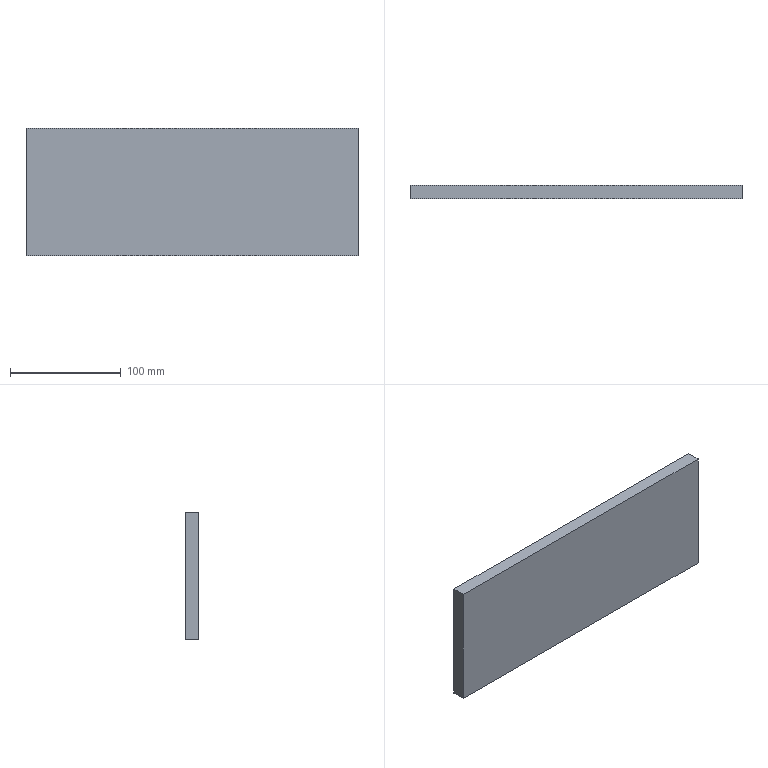Part | SolidWorks | features Extrusion 1 | 1 solid | 6 faces | box 300 x 12 x 115 mm | volume 414000 mm3 | plane 6
STEP:
#1=CARTESIAN_POINT('',(150.,0.,57.5));
#2=VERTEX_POINT('',#1);
#3=CARTESIAN_POINT('',(150.,0.,-57.5));
#4=VERTEX_POINT('',#3);
#5=CARTESIAN_POINT('',(150.,0.,57.5));
#6=DIRECTION('',(0.,0.,-1.));
#7=VECTOR('',#6,1000.);
#8=LINE('',#5,#7);
#9=EDGE_CURVE('',#2,#4,#8,.T.);
#10=ORIENTED_EDGE('',*,*,#9,.T.);
#11=CARTESIAN_POINT('',(150.,12.,-57.5));
#12=VERTEX_POINT('',#11);
#13=CARTESIAN_POINT('',(150.,12.,-57.5));
#14=DIRECTION('',(0.,-1.,0.));
#15=VECTOR('',#14,1000.);
#16=LINE('',#13,#15);
#17=EDGE_CURVE('',#12,#4,#16,.T.);
#18=ORIENTED_EDGE('',*,*,#17,.F.);
#19=CARTESIAN_POINT('',(150.,12.,57.5));
#20=VERTEX_POINT('',#19);
#21=CARTESIAN_POINT('',(150.,12.,57.5));
#22=DIRECTION('',(0.,0.,-1.));
#23=VECTOR('',#22,1000.);
#24=LINE('',#21,#23);
#25=EDGE_CURVE('',#20,#12,#24,.T.);
#26=ORIENTED_EDGE('',*,*,#25,.F.);
#27=CARTESIAN_POINT('',(150.,12.,57.5));
#28=DIRECTION('',(0.,-1.,0.));
#29=VECTOR('',#28,1000.);
#30=LINE('',#27,#29);
#31=EDGE_CURVE('',#20,#2,#30,.T.);
#32=ORIENTED_EDGE('',*,*,#31,.T.);
#33=EDGE_LOOP('',(#10,#18,#26,#32));
#34=FACE_OUTER_BOUND('',#33,.T.);
#35=CARTESIAN_POINT('',(150.,12.,57.5));
#36=DIRECTION('',(-1.,0.,0.));
#37=DIRECTION('',(0.,0.,1.));
#38=AXIS2_PLACEMENT_3D('',#35,#36,#37);
#39=PLANE('',#38);
#40=ADVANCED_FACE('',(#34),#39,.F.);
#41=CARTESIAN_POINT('',(-150.,0.,-57.5));
#42=VERTEX_POINT('',#41);
#43=CARTESIAN_POINT('',(-150.,0.,-57.5));
#44=DIRECTION('',(-1.,0.,0.));
#45=VECTOR('',#44,1000.);
#46=LINE('',#43,#45);
#47=EDGE_CURVE('',#4,#42,#46,.T.);
#48=ORIENTED_EDGE('',*,*,#47,.T.);
#49=CARTESIAN_POINT('',(-150.,12.,-57.5));
#50=VERTEX_POINT('',#49);
#51=CARTESIAN_POINT('',(-150.,12.,-57.5));
#52=DIRECTION('',(0.,-1.,0.));
#53=VECTOR('',#52,1000.);
#54=LINE('',#51,#53);
#55=EDGE_CURVE('',#50,#42,#54,.T.);
#56=ORIENTED_EDGE('',*,*,#55,.F.);
#57=CARTESIAN_POINT('',(-150.,12.,-57.5));
#58=DIRECTION('',(-1.,0.,0.));
#59=VECTOR('',#58,1000.);
#60=LINE('',#57,#59);
#61=EDGE_CURVE('',#12,#50,#60,.T.);
#62=ORIENTED_EDGE('',*,*,#61,.F.);
#63=ORIENTED_EDGE('',*,*,#17,.T.);
#64=EDGE_LOOP('',(#48,#56,#62,#63));
#65=FACE_OUTER_BOUND('',#64,.T.);
#66=CARTESIAN_POINT('',(-150.,12.,-57.5));
#67=DIRECTION('',(0.,0.,1.));
#68=DIRECTION('',(1.,0.,0.));
#69=AXIS2_PLACEMENT_3D('',#66,#67,#68);
#70=PLANE('',#69);
#71=ADVANCED_FACE('',(#65),#70,.F.);
#72=CARTESIAN_POINT('',(-150.,0.,57.5));
#73=VERTEX_POINT('',#72);
#74=CARTESIAN_POINT('',(-150.,0.,57.5));
#75=DIRECTION('',(0.,0.,1.));
#76=VECTOR('',#75,1000.);
#77=LINE('',#74,#76);
#78=EDGE_CURVE('',#42,#73,#77,.T.);
#79=ORIENTED_EDGE('',*,*,#78,.T.);
#80=CARTESIAN_POINT('',(-150.,12.,57.5));
#81=VERTEX_POINT('',#80);
#82=CARTESIAN_POINT('',(-150.,12.,57.5));
#83=DIRECTION('',(0.,-1.,0.));
#84=VECTOR('',#83,1000.);
#85=LINE('',#82,#84);
#86=EDGE_CURVE('',#81,#73,#85,.T.);
#87=ORIENTED_EDGE('',*,*,#86,.F.);
#88=CARTESIAN_POINT('',(-150.,12.,57.5));
#89=DIRECTION('',(0.,0.,1.));
#90=VECTOR('',#89,1000.);
#91=LINE('',#88,#90);
#92=EDGE_CURVE('',#50,#81,#91,.T.);
#93=ORIENTED_EDGE('',*,*,#92,.F.);
#94=ORIENTED_EDGE('',*,*,#55,.T.);
#95=EDGE_LOOP('',(#79,#87,#93,#94));
#96=FACE_OUTER_BOUND('',#95,.T.);
#97=CARTESIAN_POINT('',(-150.,12.,57.5));
#98=DIRECTION('',(1.,0.,0.));
#99=DIRECTION('',(0.,0.,-1.));
#100=AXIS2_PLACEMENT_3D('',#97,#98,#99);
#101=PLANE('',#100);
#102=ADVANCED_FACE('',(#96),#101,.F.);
#103=CARTESIAN_POINT('',(-150.,0.,57.5));
#104=DIRECTION('',(1.,0.,0.));
#105=VECTOR('',#104,1000.);
#106=LINE('',#103,#105);
#107=EDGE_CURVE('',#73,#2,#106,.T.);
#108=ORIENTED_EDGE('',*,*,#107,.T.);
#109=ORIENTED_EDGE('',*,*,#31,.F.);
#110=CARTESIAN_POINT('',(-150.,12.,57.5));
#111=DIRECTION('',(1.,0.,0.));
#112=VECTOR('',#111,1000.);
#113=LINE('',#110,#112);
#114=EDGE_CURVE('',#81,#20,#113,.T.);
#115=ORIENTED_EDGE('',*,*,#114,.F.);
#116=ORIENTED_EDGE('',*,*,#86,.T.);
#117=EDGE_LOOP('',(#108,#109,#115,#116));
#118=FACE_OUTER_BOUND('',#117,.T.);
#119=CARTESIAN_POINT('',(-150.,12.,57.5));
#120=DIRECTION('',(0.,0.,-1.));
#121=DIRECTION('',(-1.,0.,0.));
#122=AXIS2_PLACEMENT_3D('',#119,#120,#121);
#123=PLANE('',#122);
#124=ADVANCED_FACE('',(#118),#123,.F.);
#125=ORIENTED_EDGE('',*,*,#25,.T.);
#126=ORIENTED_EDGE('',*,*,#61,.T.);
#127=ORIENTED_EDGE('',*,*,#92,.T.);
#128=ORIENTED_EDGE('',*,*,#114,.T.);
#129=EDGE_LOOP('',(#125,#126,#127,#128));
#130=FACE_OUTER_BOUND('',#129,.T.);
#131=CARTESIAN_POINT('',(0.,12.,0.));
#132=DIRECTION('',(0.,-1.,0.));
#133=DIRECTION('',(0.,0.,-1.));
#134=AXIS2_PLACEMENT_3D('',#131,#132,#133);
#135=PLANE('',#134);
#136=ADVANCED_FACE('',(#130),#135,.F.);
#137=ORIENTED_EDGE('',*,*,#9,.F.);
#138=ORIENTED_EDGE('',*,*,#107,.F.);
#139=ORIENTED_EDGE('',*,*,#78,.F.);
#140=ORIENTED_EDGE('',*,*,#47,.F.);
#141=EDGE_LOOP('',(#137,#138,#139,#140));
#142=FACE_OUTER_BOUND('',#141,.T.);
#143=CARTESIAN_POINT('',(0.,0.,0.));
#144=DIRECTION('',(0.,-1.,0.));
#145=DIRECTION('',(0.,0.,-1.));
#146=AXIS2_PLACEMENT_3D('',#143,#144,#145);
#147=PLANE('',#146);
#148=ADVANCED_FACE('',(#142),#147,.T.);
#149=CLOSED_SHELL('',(#40,#71,#102,#124,#136,#148));
#150=MANIFOLD_SOLID_BREP('',#149);
#151=CARTESIAN_POINT('',(0.,0.,0.));
#152=DIRECTION('',(0.,0.,1.));
#153=DIRECTION('',(1.,0.,0.));
#154=AXIS2_PLACEMENT_3D('',#151,#152,#153);
#155=(LENGTH_UNIT()NAMED_UNIT(*)SI_UNIT(.MILLI.,.METRE.));
#156=UNCERTAINTY_MEASURE_WITH_UNIT(LENGTH_MEASURE(0.00001),#155,'','');
#157=(NAMED_UNIT(*)PLANE_ANGLE_UNIT()SI_UNIT($,.RADIAN.));
#158=(NAMED_UNIT(*)SI_UNIT($,.STERADIAN.)SOLID_ANGLE_UNIT());
#159=(GEOMETRIC_REPRESENTATION_CONTEXT(3)GLOBAL_UNCERTAINTY_ASSIGNED_CONTEXT((#156))GLOBAL_UNIT_ASSIGNED_CONTEXT((#155,#157,#158))REPRESENTATION_CONTEXT('',''));
#160=ADVANCED_BREP_SHAPE_REPRESENTATION('',(#150,#154),#159);